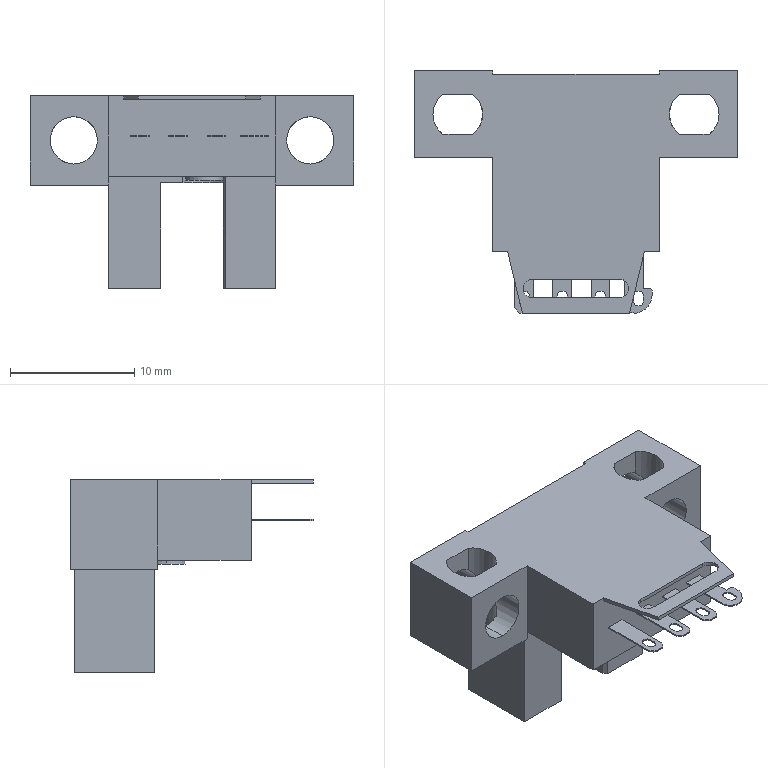Part | STEP file | 0243_014_FPML54 | 1 solid | 114 faces | box 26 x 19.5 x 15.5 mm | volume 2134 mm3 | plane 73 | cylinder 41 | commonest cylinder face diameters 0.8 x8 3.8 x8 1.5 x7 1.7 x7 4 x7 3 x3